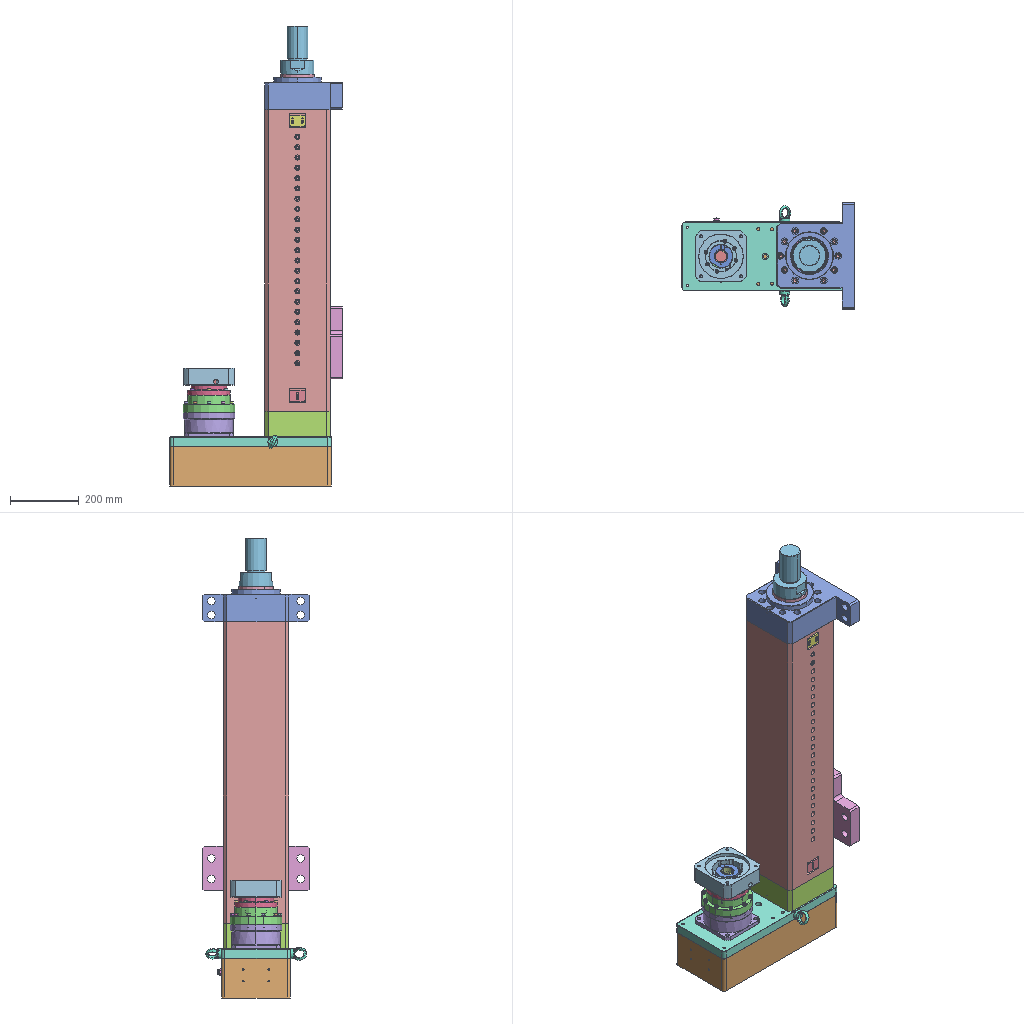Assembly | SolidWorks | 27 different items | 32 placed | box 502 x 310 x 1341 mm
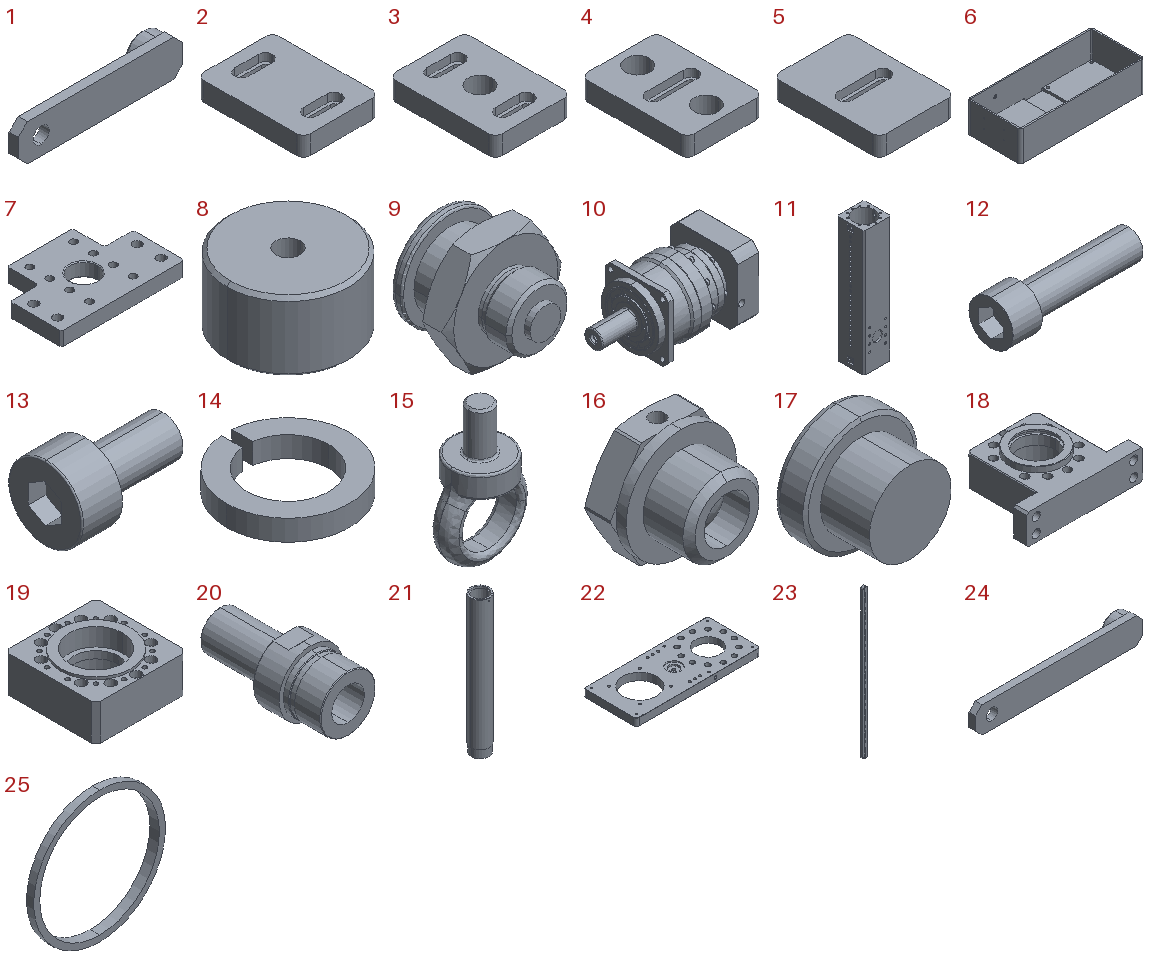Parts list (item | name | quantity | size | volume | features):
1 | - | x2 | 36 x 5 x 8 mm | 688.543 mm3 | features Chamfer 2, ICE 2, Extrusion 1
2 | - | x1 | 32 x 45 x 8 mm | 10456 mm3 | features ICE 2, Extrusion 1, Fillet 1
3 | - | x1 | 32 x 45 x 8 mm | 9802 mm3 | features ICE 2, Extrusion 1, Fillet 1, HoleWzd 1
4 | - | x1 | 32 x 45 x 8 mm | 9432 mm3 | features HoleWzd 2, ICE 2, Extrusion 1, Fillet 1
5 | - | x1 | 32 x 45 x 8 mm | 10740 mm3 | features HoleWzd 2, ICE 2, Extrusion 1, Fillet 1
6 | - | x1 | 470.5 x 201 x 115 mm | 1931028 mm3 | features ICE 4, Fillet 3, Extrusion 1, HoleWzd 1, Shell 1
7 | - | x1 | 310 x 210 x 35 mm | 1574562 mm3 | features ICE 5, Chamfer 3, Fillet 2, HoleWzd 2, Extrusion 1
8 | - | x1 | 70 x 70 x 40 mm | 146918 mm3 | features Chamfer 1, Extrusion 1, HoleWzd 1
9 | - | x1 | 19.63 x 18 x 17 mm | 2444 mm3 | features ICE 3, Revolution 2
10 | - | x1 | 297 x 150 x 150 mm | 3232491 mm3 | features BaseBody 52
11 | - | x1 | 190 x 190 x 879 mm | 15737206 mm3 | features ICE 10, HoleWzd 8, Chamfer 4, Fillet 2, LPattern 2, MirrorPattern 2, CirPattern 1, Extrusion 1
12 | - | x1 | 57 x 18 x 18 mm | 7611 mm3 | features BlendCut 1, Cut 1, Fillet 1, LPattern 1, RevCut 1, Revolution 1
13 | - | x2 | 9 x 5.5 x 5.5 mm | 106.317 mm3 | features BlendCut 1, Cut 1, Fillet 1, LPattern 1, RevCut 1, Revolution 1
14 | - | x1 | 18.367 x 18.334 x 3.1 mm | 444.091 mm3 | features Extrusion 1
15 | - | x2 | 41.795 x 29.1 x 68.897 mm | 16269 mm3 | features BaseBody 1
16 | - | x2 | 16 x 12 x 14.5 mm | 1277 mm3 | features BaseBody 1
17 | - | x1 | 14 x 9.5 x 14 mm | 897.832 mm3 | features ICE 2, Chamfer 1, Extrusion 1
18 | - | x1 | 310 x 225 x 105 mm | 2847802 mm3 | features ICE 16, Chamfer 5, HoleWzd 4, CirPattern 2, MirrorPattern 2, Extrusion 1, Fillet 1
19 | - | x1 | 190 x 190 x 90 mm | 1988671 mm3 | features ICE 14, Chamfer 4, HoleWzd 4, CirPattern 3, Extrusion 1
20 | - | x1 | 98 x 197 x 98 mm | 798757 mm3 | features ICE 11, Chamfer 1, Extrusion 1
21 | - | x1 | 100 x 100 x 741 mm | 2034515 mm3 | features ICE 6, Chamfer 2, Extrusion 1, HoleWzd 1
22 | - | x1 | 470.5 x 201 x 28 mm | 1919904 mm3 | features HoleWzd 7, ICE 7, MirrorPattern 3, Chamfer 2, Fillet 2, CirPattern 1, Extrusion 1
23 | - | x1 | 20 x 11 x 700 mm | 140963 mm3 | features Extrusion 1, Fillet 1, HoleWzd 1, ICE 1, LPattern 1, MirrorPattern 1
24 | - | x2 | 51 x 5 x 8 mm | 928.543 mm3 | features Chamfer 2, ICE 2, Extrusion 1
25 | - | x1 | 110 x 8 x 110 mm | 10853 mm3 | features Extrusion 1, ICE 1
26 | circlips for holes--type a gb | x1 | - | - | -
27 | hexagon socket head cap screws gb | x1 | - | - | -
Mates (type | each side: item.copy, entity, surface, feature):
Parallel | 11.1 face plane Boss-Extrude1 | assembly plane
Concentric | 11.1 face cylinder Boss-Extrude1 | 18.1 face cylinder Cut-Extrude1
Concentric | 11.1 face cylinder CirPattern1 | 18.1 face cylinder CirPattern1
Coincident | 11.1 face plane Boss-Extrude1 | 18.1 face plane Boss-Extrude1
Concentric | 11.1 face cylinder Boss-Extrude1 | 19.1 face cylinder Cut-Extrude11
Concentric | 11.1 face cylinder Mirror1 | 19.1 face cylinder CirPattern1
Coincident | 11.1 face plane Boss-Extrude1 | 19.1 face plane Boss-Extrude1 | 2 times
Coincident | 11.1 face plane Boss-Extrude1 | 7.1 face plane Cut-Extrude4
Concentric | 19.1 face cylinder Boss-Extrude3 | 22.1 face cylinder Cut-Extrude3
Parallel | 19.1 face plane Boss-Extrude1 | 22.1 face plane Boss-Extrude1
Coincident | 19.1 face plane Boss-Extrude1 | 22.1 face plane Boss-Extrude1
Concentric | 22.1 face cylinder Cut-Extrude1 | 10.1 face cylinder _X2_4e007ea79f7f570852a051fa8f74_X0_KS142_X2_59165f6256fe_X0_-1-solid1
Concentric | 22.1 face cylinder M10 Tapped Hole6 | 10.1 face cylinder _X2_4e007ea79f7f570852a051fa8f74_X0_KS142_X2_59165f6256fe_X0_-1-solid1
Coincident | 22.1 face plane Boss-Extrude1 | 10.1 face plane _X2_4e007ea79f7f570852a051fa8f74_X0_KS142_X2_59165f6256fe_X0_-1-solid1
Concentric | 22.1 face cylinder M12 Tapped Hole3 | 15.1 face cylinder Input1
Coincident | 6.1 face plane Boss-Extrude1 | 15.1 face plane Input1
Coincident | 6.1 face plane Boss-Extrude1 | 15.2 face plane Input1
Concentric | 11.1 face cylinder M10x1.0 Tapped Hole2 | 16.1 face cylinder Input1
Coincident | 11.1 face plane Cut-Extrude8 | 16.1 face plane Input1
Concentric | 11.1 face cylinder M10x1.0 Tapped Hole2 | 16.2 face cylinder Input1
Coincident | 11.1 face plane Cut-Extrude8 | 16.2 face plane Input1
Concentric | 11.1 face cylinder M10x1.0 Tapped Hole1 | 17.1 face cylinder Boss-Extrude1
Coincident | 11.1 face plane Cut-Extrude5 | 17.1 face plane Boss-Extrude2
Concentric | 6.1 face cylinder Cut-Extrude4 | 9.1 face cylinder Revolve1
Coincident | 6.1 face plane Boss-Extrude1 | 9.1 face plane Revolve1
Concentric | 18.1 face cylinder Cut-Extrude1 | 21.1 face cylinder Boss-Extrude1
LimitDistanceDim | 21.1 face plane Boss-Extrude1 | 18.1 face plane Boss-Extrude1
Concentric | 21.1 face cylinder Cut-Extrude10 | 20.1 face cylinder Boss-Extrude5
Coincident | 21.1 face plane Boss-Extrude1 | 20.1 face plane Boss-Extrude1
Concentric | 11.1 face cylinder Cut-Extrude10 | 7.1 face cylinder Cut-Extrude5
Parallel | 11.1 face plane Boss-Extrude1 | 7.1 face plane Boss-Extrude1
Slot | 2.1 face plane Cut-Extrude1 | 11.1 face cylinder M3 Tapped Hole2 | 2 times
Coincident | 11.1 face plane Cut-Extrude7 | 2.1 face plane Boss-Extrude1
Concentric | 10.1 face cylinder _X2_4e007ea79f7f570852a051fa8f74_X0_KS142_X2_59165f6256fe_X0_-1-solid1 | assembly face
Concentric | 7.1 face cylinder Cut-Extrude5 | 8.1 face cylinder Boss-Extrude1
Coincident | 11.1 face plane Cut-Extrude10 | 8.1 face plane Boss-Extrude1
Coincident | 18.1 face plane Cut-Extrude7 | 25.1 face plane Boss-Extrude1
Concentric | 12.1 face cylinder Base-Revolve | 14.1 face cylinder Extrude1
Coincident | 12.1 face plane Base-Revolve | 14.1 face plane Extrude1
Parallel | 24.1 face plane Boss-Extrude1 | 1.1 face plane Boss-Extrude1
Slot | 3.1 face plane Cut-Extrude1 | 11.1 face cylinder M3 Tapped Hole2 | 2 times
Coincident | 11.1 face plane Mirror2 | 3.1 face plane Boss-Extrude1
Slot | 4.1 face cylinder M12 Tapped Hole2 | 11.1 face plane Cut-Extrude3 | 2 times
Coincident | 11.1 face plane Mirror2 | 4.1 face plane Boss-Extrude1
Concentric | 11.1 face cylinder M3 Tapped Hole3 | 13.1 face cylinder Base-Revolve
Coincident | 4.1 face plane Cut-Extrude2 | 13.1 face plane Base-Revolve
Concentric | 11.1 face cylinder M3 Tapped Hole3 | 13.2 face cylinder Base-Revolve
Coincident | 13.1 face plane Base-Revolve | 13.2 face plane Base-Revolve
Coincident | 11.1 face plane Cut-Extrude6 | 5.1 face plane Boss-Extrude1
DistanceDim | 5.1 face plane Boss-Extrude1 | 11.1 face plane Cut-Extrude6 | 2 times
Tangent | 11.1 face cylinder Boss-Extrude1 | 23.1 face plane Boss-Extrude1
Concentric | 11.1 face cylinder Cut-Extrude1 | 23.1 face cylinder LPattern1
Concentric | 11.1 face cylinder LPattern1 | 23.1 face cylinder LPattern1
Coincident | 22.1 face plane Boss-Extrude1 | 6.1 face plane Boss-Extrude1 | 2 times
Concentric | 22.1 face cylinder Mirror7 | 15.2 face cylinder Input1
Coincident | 22.1 face plane Boss-Extrude1 | 15.2 face plane Input1
Parallel | 18.1 face plane Boss-Extrude1 | 20.1 face plane Cut-Extrude1